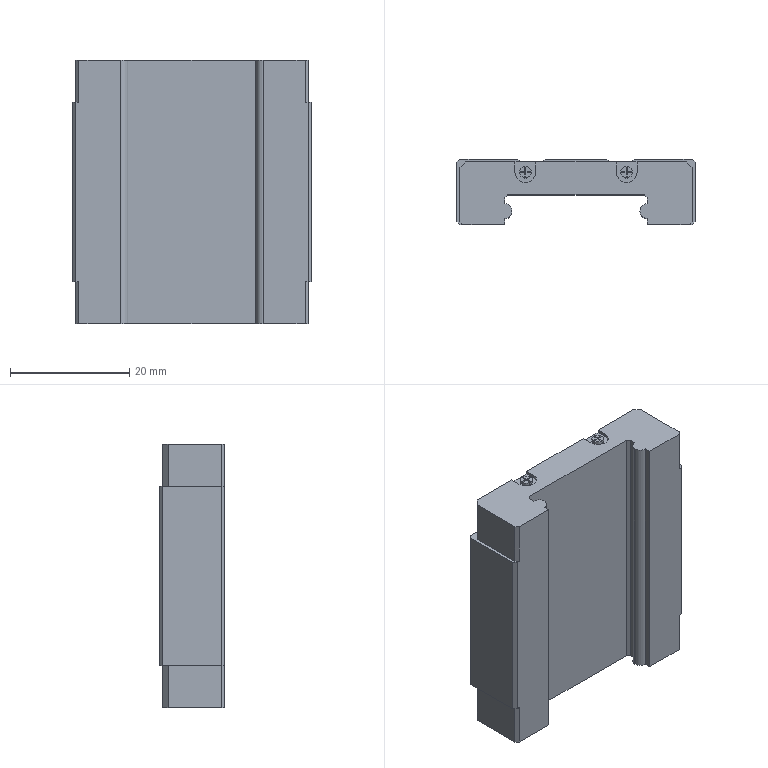Part | STEP file | block_SEBWN14 | 1 solid | 159 faces | box 40 x 11 x 44.3 mm | volume 13647 mm3 | plane 115 | cylinder 28 | cone 16 | commonest cylinder face diameters 2 x8 2.459 x8 3 x5 3.5 x4 2.5 x3